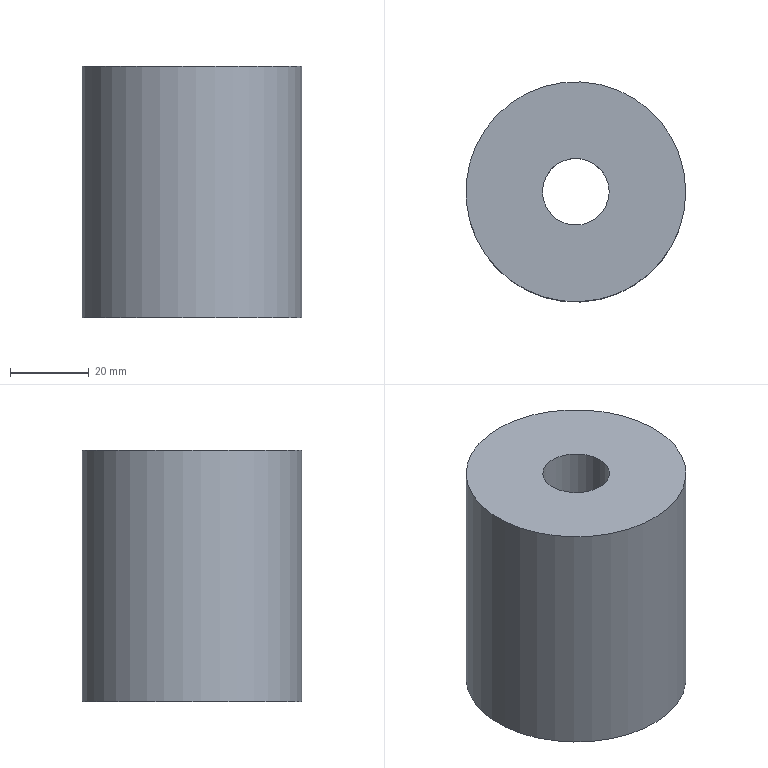Part | NX | 1 solid | 6 faces | box 56 x 56 x 64 mm | volume 141296 mm3 | cylinder 3 | plane 3 | commonest cylinder face diameters 17 x1 19 x1 56 x1
STEP:
#1=CARTESIAN_POINT('',(28.,0.,64.));
#2=VERTEX_POINT('',#1);
#3=CARTESIAN_POINT('',(0.,0.,64.));
#4=DIRECTION('',(0.,0.,1.));
#5=DIRECTION('',(1.,0.,0.));
#6=AXIS2_PLACEMENT_3D('',#3,#4,#5);
#7=CIRCLE('',#6,28.);
#8=EDGE_CURVE('',#2,#2,#7,.T.);
#9=ORIENTED_EDGE('',*,*,#8,.F.);
#10=EDGE_LOOP('',(#9));
#11=FACE_BOUND('',#10,.T.);
#12=CARTESIAN_POINT('',(28.,0.,0.));
#13=VERTEX_POINT('',#12);
#14=CARTESIAN_POINT('',(0.,0.,0.));
#15=DIRECTION('',(0.,0.,1.));
#16=DIRECTION('',(1.,0.,0.));
#17=AXIS2_PLACEMENT_3D('',#14,#15,#16);
#18=CIRCLE('',#17,28.);
#19=EDGE_CURVE('',#13,#13,#18,.T.);
#20=ORIENTED_EDGE('',*,*,#19,.T.);
#21=EDGE_LOOP('',(#20));
#22=FACE_BOUND('',#21,.T.);
#23=CARTESIAN_POINT('',(0.,0.,64.));
#24=DIRECTION('',(0.,0.,-1.));
#25=DIRECTION('',(-1.,0.,0.));
#26=AXIS2_PLACEMENT_3D('',#23,#24,#25);
#27=CYLINDRICAL_SURFACE('',#26,28.);
#28=ADVANCED_FACE('',(#11,#22),#27,.T.);
#29=CARTESIAN_POINT('',(8.5,0.,64.));
#30=VERTEX_POINT('',#29);
#31=CARTESIAN_POINT('',(0.,0.,64.));
#32=DIRECTION('',(0.,0.,1.));
#33=DIRECTION('',(1.,0.,0.));
#34=AXIS2_PLACEMENT_3D('',#31,#32,#33);
#35=CIRCLE('',#34,8.5);
#36=EDGE_CURVE('',#30,#30,#35,.T.);
#37=ORIENTED_EDGE('',*,*,#36,.F.);
#38=EDGE_LOOP('',(#37));
#39=FACE_BOUND('',#38,.T.);
#40=ORIENTED_EDGE('',*,*,#8,.T.);
#41=EDGE_LOOP('',(#40));
#42=FACE_BOUND('',#41,.T.);
#43=CARTESIAN_POINT('',(0.,0.,64.));
#44=DIRECTION('',(0.,0.,1.));
#45=DIRECTION('',(1.,0.,0.));
#46=AXIS2_PLACEMENT_3D('',#43,#44,#45);
#47=PLANE('',#46);
#48=ADVANCED_FACE('',(#39,#42),#47,.T.);
#49=CARTESIAN_POINT('',(-9.5,0.,0.));
#50=VERTEX_POINT('',#49);
#51=CARTESIAN_POINT('',(0.,0.,0.));
#52=DIRECTION('',(0.,0.,-1.));
#53=DIRECTION('',(-1.,0.,0.));
#54=AXIS2_PLACEMENT_3D('',#51,#52,#53);
#55=CIRCLE('',#54,9.5);
#56=EDGE_CURVE('',#50,#50,#55,.T.);
#57=ORIENTED_EDGE('',*,*,#56,.F.);
#58=EDGE_LOOP('',(#57));
#59=FACE_BOUND('',#58,.T.);
#60=ORIENTED_EDGE('',*,*,#19,.F.);
#61=EDGE_LOOP('',(#60));
#62=FACE_BOUND('',#61,.T.);
#63=CARTESIAN_POINT('',(0.,0.,0.));
#64=DIRECTION('',(0.,0.,1.));
#65=DIRECTION('',(1.,0.,0.));
#66=AXIS2_PLACEMENT_3D('',#63,#64,#65);
#67=PLANE('',#66);
#68=ADVANCED_FACE('',(#59,#62),#67,.F.);
#69=CARTESIAN_POINT('',(-8.5,0.,32.));
#70=VERTEX_POINT('',#69);
#71=CARTESIAN_POINT('',(0.,0.,32.));
#72=DIRECTION('',(0.,0.,-1.));
#73=DIRECTION('',(-1.,0.,0.));
#74=AXIS2_PLACEMENT_3D('',#71,#72,#73);
#75=CIRCLE('',#74,8.5);
#76=EDGE_CURVE('',#70,#70,#75,.F.);
#77=ORIENTED_EDGE('',*,*,#76,.F.);
#78=EDGE_LOOP('',(#77));
#79=FACE_BOUND('',#78,.T.);
#80=ORIENTED_EDGE('',*,*,#36,.T.);
#81=EDGE_LOOP('',(#80));
#82=FACE_BOUND('',#81,.T.);
#83=CARTESIAN_POINT('',(0.,0.,32.));
#84=DIRECTION('',(0.,0.,1.));
#85=DIRECTION('',(1.,0.,0.));
#86=AXIS2_PLACEMENT_3D('',#83,#84,#85);
#87=CYLINDRICAL_SURFACE('',#86,8.5);
#88=ADVANCED_FACE('',(#79,#82),#87,.F.);
#89=CARTESIAN_POINT('',(-9.5,0.,32.));
#90=VERTEX_POINT('',#89);
#91=CARTESIAN_POINT('',(0.,0.,32.));
#92=DIRECTION('',(0.,0.,-1.));
#93=DIRECTION('',(-1.,0.,0.));
#94=AXIS2_PLACEMENT_3D('',#91,#92,#93);
#95=CIRCLE('',#94,9.5);
#96=EDGE_CURVE('',#90,#90,#95,.T.);
#97=ORIENTED_EDGE('',*,*,#96,.T.);
#98=EDGE_LOOP('',(#97));
#99=FACE_BOUND('',#98,.T.);
#100=ORIENTED_EDGE('',*,*,#76,.T.);
#101=EDGE_LOOP('',(#100));
#102=FACE_BOUND('',#101,.T.);
#103=CARTESIAN_POINT('',(0.,0.,32.));
#104=DIRECTION('',(0.,0.,-1.));
#105=DIRECTION('',(-1.,0.,0.));
#106=AXIS2_PLACEMENT_3D('',#103,#104,#105);
#107=PLANE('',#106);
#108=ADVANCED_FACE('',(#99,#102),#107,.T.);
#109=ORIENTED_EDGE('',*,*,#96,.F.);
#110=EDGE_LOOP('',(#109));
#111=FACE_BOUND('',#110,.T.);
#112=ORIENTED_EDGE('',*,*,#56,.T.);
#113=EDGE_LOOP('',(#112));
#114=FACE_BOUND('',#113,.T.);
#115=CARTESIAN_POINT('',(0.,0.,32.));
#116=DIRECTION('',(0.,0.,-1.));
#117=DIRECTION('',(-1.,0.,0.));
#118=AXIS2_PLACEMENT_3D('',#115,#116,#117);
#119=CYLINDRICAL_SURFACE('',#118,9.5);
#120=ADVANCED_FACE('',(#111,#114),#119,.F.);
#121=CLOSED_SHELL('',(#28,#48,#68,#88,#108,#120));
#122=MANIFOLD_SOLID_BREP('',#121);
#123=(LENGTH_UNIT()NAMED_UNIT(*)SI_UNIT(.MILLI.,.METRE.));
#124=UNCERTAINTY_MEASURE_WITH_UNIT(LENGTH_MEASURE(0.00001),#123,'','');
#125=(NAMED_UNIT(*)PLANE_ANGLE_UNIT()SI_UNIT($,.RADIAN.));
#126=(NAMED_UNIT(*)SI_UNIT($,.STERADIAN.)SOLID_ANGLE_UNIT());
#127=(GEOMETRIC_REPRESENTATION_CONTEXT(3)GLOBAL_UNCERTAINTY_ASSIGNED_CONTEXT((#124))GLOBAL_UNIT_ASSIGNED_CONTEXT((#123,#125,#126))REPRESENTATION_CONTEXT('',''));
#128=ADVANCED_BREP_SHAPE_REPRESENTATION('',(#122),#127);